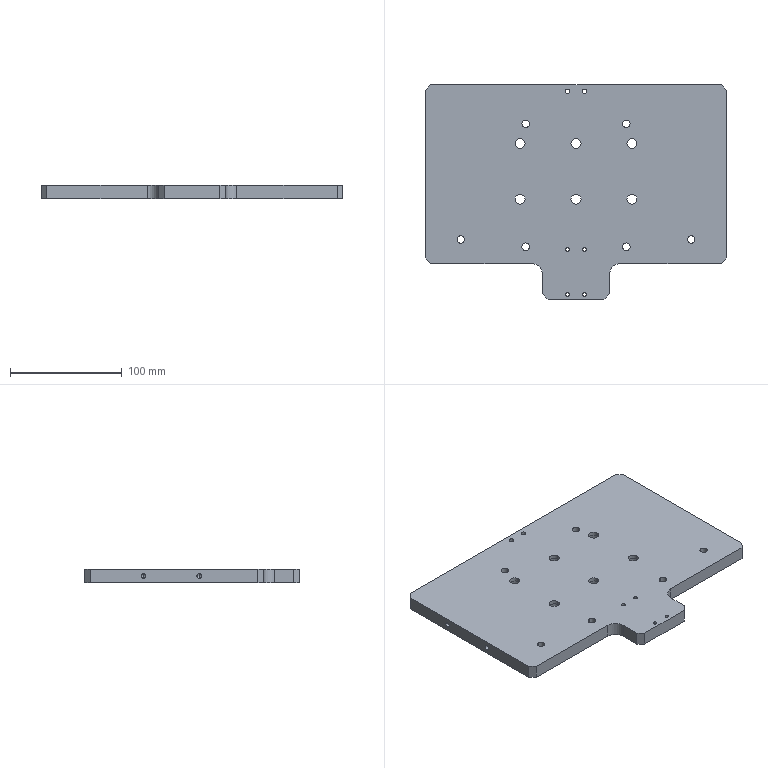Part | SolidWorks | features HoleWzd 8, Chamfer 1, Extrusion 1, Fillet 1, ICE 1, MirrorPattern 1 | 1 solid | 88 faces | box 270 x 192 x 12 mm | volume 526570 mm3 | cylinder 58 | plane 22 | cone 8 | commonest cylinder face diameters 4.2 x12 6.8 x12 9 x12 15 x12 3.3 x8 20 x2